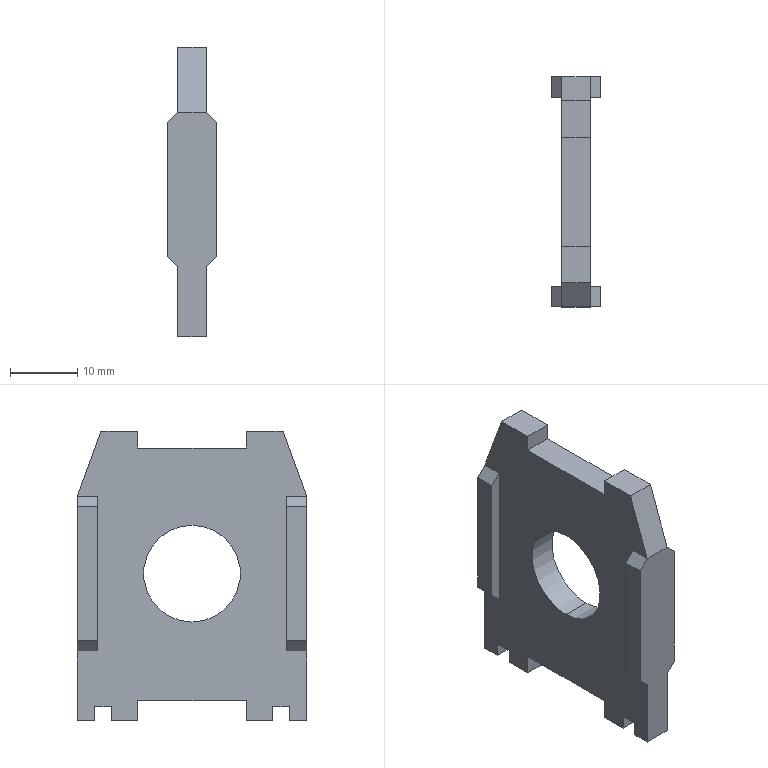Part | STEP file | 11-GY_Y300T-A_SCREW-30-V10-22111.11 | 1 solid | 42 faces | box 7.2 x 34.2 x 43.1 mm | volume 5332 mm3 | plane 40 | cylinder 2 | commonest cylinder face diameters 14.4 x2
STEP:
#1=CARTESIAN_POINT('',(-2.1,0.,7.2));
#2=VERTEX_POINT('',#1);
#3=CARTESIAN_POINT('',(-2.1,0.,-7.2));
#4=VERTEX_POINT('',#3);
#5=CARTESIAN_POINT('',(-2.1,0.,0.));
#6=DIRECTION('',(1.,0.,0.));
#7=DIRECTION('',(0.,0.,-1.));
#8=AXIS2_PLACEMENT_3D('',#5,#6,#7);
#9=CIRCLE('',#8,7.2);
#10=EDGE_CURVE('',#2,#4,#9,.T.);
#11=ORIENTED_EDGE('',*,*,#10,.F.);
#12=CARTESIAN_POINT('',(2.1,0.,7.2));
#13=VERTEX_POINT('',#12);
#14=CARTESIAN_POINT('',(2.1,0.,7.2));
#15=DIRECTION('',(1.,0.,0.));
#16=VECTOR('',#15,1000.);
#17=LINE('',#14,#16);
#18=EDGE_CURVE('',#2,#13,#17,.T.);
#19=ORIENTED_EDGE('',*,*,#18,.T.);
#20=CARTESIAN_POINT('',(2.1,0.,-7.2));
#21=VERTEX_POINT('',#20);
#22=CARTESIAN_POINT('',(2.1,0.,0.));
#23=DIRECTION('',(-1.,0.,0.));
#24=DIRECTION('',(0.,0.,-1.));
#25=AXIS2_PLACEMENT_3D('',#22,#23,#24);
#26=CIRCLE('',#25,7.2);
#27=EDGE_CURVE('',#21,#13,#26,.T.);
#28=ORIENTED_EDGE('',*,*,#27,.F.);
#29=CARTESIAN_POINT('',(2.1,0.,-7.2));
#30=DIRECTION('',(1.,0.,0.));
#31=VECTOR('',#30,1000.);
#32=LINE('',#29,#31);
#33=EDGE_CURVE('',#4,#21,#32,.T.);
#34=ORIENTED_EDGE('',*,*,#33,.F.);
#35=EDGE_LOOP('',(#11,#19,#28,#34));
#36=FACE_OUTER_BOUND('',#35,.T.);
#37=CARTESIAN_POINT('',(2.1,0.,0.));
#38=DIRECTION('',(1.,0.,0.));
#39=DIRECTION('',(0.,0.,-1.));
#40=AXIS2_PLACEMENT_3D('',#37,#38,#39);
#41=CYLINDRICAL_SURFACE('',#40,7.2);
#42=ADVANCED_FACE('',(#36),#41,.F.);
#43=CARTESIAN_POINT('',(2.1,-8.1,18.7));
#44=VERTEX_POINT('',#43);
#45=CARTESIAN_POINT('',(2.1,-8.1,21.2));
#46=VERTEX_POINT('',#45);
#47=CARTESIAN_POINT('',(2.1,-8.1,0.));
#48=DIRECTION('',(0.,0.,1.));
#49=VECTOR('',#48,1000.);
#50=LINE('',#47,#49);
#51=EDGE_CURVE('',#44,#46,#50,.T.);
#52=ORIENTED_EDGE('',*,*,#51,.T.);
#53=CARTESIAN_POINT('',(2.1,-13.569,21.2));
#54=VERTEX_POINT('',#53);
#55=CARTESIAN_POINT('',(2.1,0.,21.2));
#56=DIRECTION('',(0.,-1.,0.));
#57=VECTOR('',#56,1000.);
#58=LINE('',#55,#57);
#59=EDGE_CURVE('',#46,#54,#58,.T.);
#60=ORIENTED_EDGE('',*,*,#59,.T.);
#61=CARTESIAN_POINT('',(2.1,-17.1,11.5));
#62=VERTEX_POINT('',#61);
#63=CARTESIAN_POINT('',(2.1,-13.569,21.2));
#64=DIRECTION('',(0.,-0.342,-0.9397));
#65=VECTOR('',#64,1000.);
#66=LINE('',#63,#65);
#67=EDGE_CURVE('',#54,#62,#66,.T.);
#68=ORIENTED_EDGE('',*,*,#67,.T.);
#69=CARTESIAN_POINT('',(2.1,-14.1,11.5));
#70=VERTEX_POINT('',#69);
#71=CARTESIAN_POINT('',(2.1,0.,11.5));
#72=DIRECTION('',(0.,1.,0.));
#73=VECTOR('',#72,1000.);
#74=LINE('',#71,#73);
#75=EDGE_CURVE('',#62,#70,#74,.T.);
#76=ORIENTED_EDGE('',*,*,#75,.T.);
#77=CARTESIAN_POINT('',(2.1,-14.1,-11.5));
#78=VERTEX_POINT('',#77);
#79=CARTESIAN_POINT('',(2.1,-14.1,0.));
#80=DIRECTION('',(0.,0.,-1.));
#81=VECTOR('',#80,1000.);
#82=LINE('',#79,#81);
#83=EDGE_CURVE('',#70,#78,#82,.T.);
#84=ORIENTED_EDGE('',*,*,#83,.T.);
#85=CARTESIAN_POINT('',(2.1,-17.1,-11.5));
#86=VERTEX_POINT('',#85);
#87=CARTESIAN_POINT('',(2.1,0.,-11.5));
#88=DIRECTION('',(0.,-1.,0.));
#89=VECTOR('',#88,1000.);
#90=LINE('',#87,#89);
#91=EDGE_CURVE('',#78,#86,#90,.T.);
#92=ORIENTED_EDGE('',*,*,#91,.T.);
#93=CARTESIAN_POINT('',(2.1,-17.1,-21.9));
#94=VERTEX_POINT('',#93);
#95=CARTESIAN_POINT('',(2.1,-17.1,0.));
#96=DIRECTION('',(0.,0.,-1.));
#97=VECTOR('',#96,1000.);
#98=LINE('',#95,#97);
#99=EDGE_CURVE('',#86,#94,#98,.T.);
#100=ORIENTED_EDGE('',*,*,#99,.T.);
#101=CARTESIAN_POINT('',(2.1,-14.5,-21.9));
#102=VERTEX_POINT('',#101);
#103=CARTESIAN_POINT('',(2.1,0.,-21.9));
#104=DIRECTION('',(0.,1.,0.));
#105=VECTOR('',#104,1000.);
#106=LINE('',#103,#105);
#107=EDGE_CURVE('',#94,#102,#106,.T.);
#108=ORIENTED_EDGE('',*,*,#107,.T.);
#109=CARTESIAN_POINT('',(2.1,-14.5,-19.8));
#110=VERTEX_POINT('',#109);
#111=CARTESIAN_POINT('',(2.1,-14.5,0.));
#112=DIRECTION('',(0.,0.,1.));
#113=VECTOR('',#112,1000.);
#114=LINE('',#111,#113);
#115=EDGE_CURVE('',#102,#110,#114,.T.);
#116=ORIENTED_EDGE('',*,*,#115,.T.);
#117=CARTESIAN_POINT('',(2.1,-12.,-19.8));
#118=VERTEX_POINT('',#117);
#119=CARTESIAN_POINT('',(2.1,0.,-19.8));
#120=DIRECTION('',(0.,1.,0.));
#121=VECTOR('',#120,1000.);
#122=LINE('',#119,#121);
#123=EDGE_CURVE('',#110,#118,#122,.T.);
#124=ORIENTED_EDGE('',*,*,#123,.T.);
#125=CARTESIAN_POINT('',(2.1,-12.,-21.9));
#126=VERTEX_POINT('',#125);
#127=CARTESIAN_POINT('',(2.1,-12.,0.));
#128=DIRECTION('',(0.,0.,-1.));
#129=VECTOR('',#128,1000.);
#130=LINE('',#127,#129);
#131=EDGE_CURVE('',#118,#126,#130,.T.);
#132=ORIENTED_EDGE('',*,*,#131,.T.);
#133=CARTESIAN_POINT('',(2.1,-8.1,-21.9));
#134=VERTEX_POINT('',#133);
#135=CARTESIAN_POINT('',(2.1,0.,-21.9));
#136=DIRECTION('',(0.,1.,0.));
#137=VECTOR('',#136,1000.);
#138=LINE('',#135,#137);
#139=EDGE_CURVE('',#126,#134,#138,.T.);
#140=ORIENTED_EDGE('',*,*,#139,.T.);
#141=CARTESIAN_POINT('',(2.1,-8.1,-18.9));
#142=VERTEX_POINT('',#141);
#143=CARTESIAN_POINT('',(2.1,-8.1,0.));
#144=DIRECTION('',(0.,0.,1.));
#145=VECTOR('',#144,1000.);
#146=LINE('',#143,#145);
#147=EDGE_CURVE('',#134,#142,#146,.T.);
#148=ORIENTED_EDGE('',*,*,#147,.T.);
#149=CARTESIAN_POINT('',(2.1,8.1,-18.9));
#150=VERTEX_POINT('',#149);
#151=CARTESIAN_POINT('',(2.1,0.,-18.9));
#152=DIRECTION('',(0.,1.,0.));
#153=VECTOR('',#152,1000.);
#154=LINE('',#151,#153);
#155=EDGE_CURVE('',#142,#150,#154,.T.);
#156=ORIENTED_EDGE('',*,*,#155,.T.);
#157=CARTESIAN_POINT('',(2.1,8.1,-21.9));
#158=VERTEX_POINT('',#157);
#159=CARTESIAN_POINT('',(2.1,8.1,0.));
#160=DIRECTION('',(0.,0.,-1.));
#161=VECTOR('',#160,1000.);
#162=LINE('',#159,#161);
#163=EDGE_CURVE('',#150,#158,#162,.T.);
#164=ORIENTED_EDGE('',*,*,#163,.T.);
#165=CARTESIAN_POINT('',(2.1,12.,-21.9));
#166=VERTEX_POINT('',#165);
#167=CARTESIAN_POINT('',(2.1,0.,-21.9));
#168=DIRECTION('',(0.,1.,0.));
#169=VECTOR('',#168,1000.);
#170=LINE('',#167,#169);
#171=EDGE_CURVE('',#158,#166,#170,.T.);
#172=ORIENTED_EDGE('',*,*,#171,.T.);
#173=CARTESIAN_POINT('',(2.1,12.,-19.8));
#174=VERTEX_POINT('',#173);
#175=CARTESIAN_POINT('',(2.1,12.,0.));
#176=DIRECTION('',(0.,0.,1.));
#177=VECTOR('',#176,1000.);
#178=LINE('',#175,#177);
#179=EDGE_CURVE('',#166,#174,#178,.T.);
#180=ORIENTED_EDGE('',*,*,#179,.T.);
#181=CARTESIAN_POINT('',(2.1,14.5,-19.8));
#182=VERTEX_POINT('',#181);
#183=CARTESIAN_POINT('',(2.1,0.,-19.8));
#184=DIRECTION('',(0.,1.,0.));
#185=VECTOR('',#184,1000.);
#186=LINE('',#183,#185);
#187=EDGE_CURVE('',#174,#182,#186,.T.);
#188=ORIENTED_EDGE('',*,*,#187,.T.);
#189=CARTESIAN_POINT('',(2.1,14.5,-21.9));
#190=VERTEX_POINT('',#189);
#191=CARTESIAN_POINT('',(2.1,14.5,0.));
#192=DIRECTION('',(0.,0.,-1.));
#193=VECTOR('',#192,1000.);
#194=LINE('',#191,#193);
#195=EDGE_CURVE('',#182,#190,#194,.T.);
#196=ORIENTED_EDGE('',*,*,#195,.T.);
#197=CARTESIAN_POINT('',(2.1,17.1,-21.9));
#198=VERTEX_POINT('',#197);
#199=CARTESIAN_POINT('',(2.1,0.,-21.9));
#200=DIRECTION('',(0.,1.,0.));
#201=VECTOR('',#200,1000.);
#202=LINE('',#199,#201);
#203=EDGE_CURVE('',#190,#198,#202,.T.);
#204=ORIENTED_EDGE('',*,*,#203,.T.);
#205=CARTESIAN_POINT('',(2.1,17.1,-11.5));
#206=VERTEX_POINT('',#205);
#207=CARTESIAN_POINT('',(2.1,17.1,0.));
#208=DIRECTION('',(0.,0.,1.));
#209=VECTOR('',#208,1000.);
#210=LINE('',#207,#209);
#211=EDGE_CURVE('',#198,#206,#210,.T.);
#212=ORIENTED_EDGE('',*,*,#211,.T.);
#213=CARTESIAN_POINT('',(2.1,14.1,-11.5));
#214=VERTEX_POINT('',#213);
#215=CARTESIAN_POINT('',(2.1,0.,-11.5));
#216=DIRECTION('',(0.,-1.,0.));
#217=VECTOR('',#216,1000.);
#218=LINE('',#215,#217);
#219=EDGE_CURVE('',#206,#214,#218,.T.);
#220=ORIENTED_EDGE('',*,*,#219,.T.);
#221=CARTESIAN_POINT('',(2.1,14.1,11.5));
#222=VERTEX_POINT('',#221);
#223=CARTESIAN_POINT('',(2.1,14.1,0.));
#224=DIRECTION('',(0.,0.,1.));
#225=VECTOR('',#224,1000.);
#226=LINE('',#223,#225);
#227=EDGE_CURVE('',#214,#222,#226,.T.);
#228=ORIENTED_EDGE('',*,*,#227,.T.);
#229=CARTESIAN_POINT('',(2.1,17.1,11.5));
#230=VERTEX_POINT('',#229);
#231=CARTESIAN_POINT('',(2.1,0.,11.5));
#232=DIRECTION('',(0.,1.,0.));
#233=VECTOR('',#232,1000.);
#234=LINE('',#231,#233);
#235=EDGE_CURVE('',#222,#230,#234,.T.);
#236=ORIENTED_EDGE('',*,*,#235,.T.);
#237=CARTESIAN_POINT('',(2.1,13.569,21.2));
#238=VERTEX_POINT('',#237);
#239=CARTESIAN_POINT('',(2.1,17.1,11.5));
#240=DIRECTION('',(0.,-0.342,0.9397));
#241=VECTOR('',#240,1000.);
#242=LINE('',#239,#241);
#243=EDGE_CURVE('',#230,#238,#242,.T.);
#244=ORIENTED_EDGE('',*,*,#243,.T.);
#245=CARTESIAN_POINT('',(2.1,8.1,21.2));
#246=VERTEX_POINT('',#245);
#247=CARTESIAN_POINT('',(2.1,0.,21.2));
#248=DIRECTION('',(0.,-1.,0.));
#249=VECTOR('',#248,1000.);
#250=LINE('',#247,#249);
#251=EDGE_CURVE('',#238,#246,#250,.T.);
#252=ORIENTED_EDGE('',*,*,#251,.T.);
#253=CARTESIAN_POINT('',(2.1,8.1,18.7));
#254=VERTEX_POINT('',#253);
#255=CARTESIAN_POINT('',(2.1,8.1,0.));
#256=DIRECTION('',(0.,0.,-1.));
#257=VECTOR('',#256,1000.);
#258=LINE('',#255,#257);
#259=EDGE_CURVE('',#246,#254,#258,.T.);
#260=ORIENTED_EDGE('',*,*,#259,.T.);
#261=CARTESIAN_POINT('',(2.1,0.,18.7));
#262=DIRECTION('',(0.,-1.,0.));
#263=VECTOR('',#262,1000.);
#264=LINE('',#261,#263);
#265=EDGE_CURVE('',#254,#44,#264,.T.);
#266=ORIENTED_EDGE('',*,*,#265,.T.);
#267=EDGE_LOOP('',(#52,#60,#68,#76,#84,#92,#100,#108,#116,#124,#132,#140,#148,#156,#164,#172,#180,#188,#196,#204,#212,#220,#228,#236,#244,#252,#260,#266));
#268=FACE_OUTER_BOUND('',#267,.T.);
#269=ORIENTED_EDGE('',*,*,#27,.T.);
#270=CARTESIAN_POINT('',(2.1,0.,0.));
#271=DIRECTION('',(-1.,0.,0.));
#272=DIRECTION('',(0.,0.,-1.));
#273=AXIS2_PLACEMENT_3D('',#270,#271,#272);
#274=CIRCLE('',#273,7.2);
#275=EDGE_CURVE('',#13,#21,#274,.T.);
#276=ORIENTED_EDGE('',*,*,#275,.T.);
#277=EDGE_LOOP('',(#269,#276));
#278=FACE_BOUND('',#277,.T.);
#279=CARTESIAN_POINT('',(2.1,0.,0.));
#280=DIRECTION('',(1.,0.,0.));
#281=DIRECTION('',(0.,0.,-1.));
#282=AXIS2_PLACEMENT_3D('',#279,#280,#281);
#283=PLANE('',#282);
#284=ADVANCED_FACE('',(#268,#278),#283,.T.);
#285=CARTESIAN_POINT('',(-2.1,-13.569,21.2));
#286=VERTEX_POINT('',#285);
#287=CARTESIAN_POINT('',(2.1,-13.569,21.2));
#288=DIRECTION('',(-1.,0.,0.));
#289=VECTOR('',#288,1000.);
#290=LINE('',#287,#289);
#291=EDGE_CURVE('',#54,#286,#290,.T.);
#292=ORIENTED_EDGE('',*,*,#291,.F.);
#293=ORIENTED_EDGE('',*,*,#59,.F.);
#294=CARTESIAN_POINT('',(-2.1,-8.1,21.2));
#295=VERTEX_POINT('',#294);
#296=CARTESIAN_POINT('',(2.1,-8.1,21.2));
#297=DIRECTION('',(1.,0.,0.));
#298=VECTOR('',#297,1000.);
#299=LINE('',#296,#298);
#300=EDGE_CURVE('',#295,#46,#299,.T.);
#301=ORIENTED_EDGE('',*,*,#300,.F.);
#302=CARTESIAN_POINT('',(-2.1,-8.1,21.2));
#303=DIRECTION('',(0.,1.,0.));
#304=VECTOR('',#303,1000.);
#305=LINE('',#302,#304);
#306=EDGE_CURVE('',#286,#295,#305,.T.);
#307=ORIENTED_EDGE('',*,*,#306,.F.);
#308=EDGE_LOOP('',(#292,#293,#301,#307));
#309=FACE_OUTER_BOUND('',#308,.T.);
#310=CARTESIAN_POINT('',(2.1,-8.1,21.2));
#311=DIRECTION('',(0.,0.,-1.));
#312=DIRECTION('',(-1.,0.,0.));
#313=AXIS2_PLACEMENT_3D('',#310,#311,#312);
#314=PLANE('',#313);
#315=ADVANCED_FACE('',(#309),#314,.F.);
#316=ORIENTED_EDGE('',*,*,#300,.T.);
#317=ORIENTED_EDGE('',*,*,#51,.F.);
#318=CARTESIAN_POINT('',(-2.1,-8.1,18.7));
#319=VERTEX_POINT('',#318);
#320=CARTESIAN_POINT('',(2.1,-8.1,18.7));
#321=DIRECTION('',(1.,0.,0.));
#322=VECTOR('',#321,1000.);
#323=LINE('',#320,#322);
#324=EDGE_CURVE('',#319,#44,#323,.T.);
#325=ORIENTED_EDGE('',*,*,#324,.F.);
#326=CARTESIAN_POINT('',(-2.1,-8.1,18.7));
#327=DIRECTION('',(0.,0.,-1.));
#328=VECTOR('',#327,1000.);
#329=LINE('',#326,#328);
#330=EDGE_CURVE('',#295,#319,#329,.T.);
#331=ORIENTED_EDGE('',*,*,#330,.F.);
#332=EDGE_LOOP('',(#316,#317,#325,#331));
#333=FACE_OUTER_BOUND('',#332,.T.);
#334=CARTESIAN_POINT('',(2.1,-8.1,18.7));
#335=DIRECTION('',(0.,-1.,0.));
#336=DIRECTION('',(0.,0.,-1.));
#337=AXIS2_PLACEMENT_3D('',#334,#335,#336);
#338=PLANE('',#337);
#339=ADVANCED_FACE('',(#333),#338,.F.);
#340=ORIENTED_EDGE('',*,*,#324,.T.);
#341=ORIENTED_EDGE('',*,*,#265,.F.);
#342=CARTESIAN_POINT('',(-2.1,8.1,18.7));
#343=VERTEX_POINT('',#342);
#344=CARTESIAN_POINT('',(2.1,8.1,18.7));
#345=DIRECTION('',(1.,0.,0.));
#346=VECTOR('',#345,1000.);
#347=LINE('',#344,#346);
#348=EDGE_CURVE('',#343,#254,#347,.T.);
#349=ORIENTED_EDGE('',*,*,#348,.F.);
#350=CARTESIAN_POINT('',(-2.1,8.1,18.7));
#351=DIRECTION('',(0.,1.,0.));
#352=VECTOR('',#351,1000.);
#353=LINE('',#350,#352);
#354=EDGE_CURVE('',#319,#343,#353,.T.);
#355=ORIENTED_EDGE('',*,*,#354,.F.);
#356=EDGE_LOOP('',(#340,#341,#349,#355));
#357=FACE_OUTER_BOUND('',#356,.T.);
#358=CARTESIAN_POINT('',(2.1,8.1,18.7));
#359=DIRECTION('',(0.,0.,-1.));
#360=DIRECTION('',(-1.,0.,0.));
#361=AXIS2_PLACEMENT_3D('',#358,#359,#360);
#362=PLANE('',#361);
#363=ADVANCED_FACE('',(#357),#362,.F.);
#364=ORIENTED_EDGE('',*,*,#348,.T.);
#365=ORIENTED_EDGE('',*,*,#259,.F.);
#366=CARTESIAN_POINT('',(-2.1,8.1,21.2));
#367=VERTEX_POINT('',#366);
#368=CARTESIAN_POINT('',(2.1,8.1,21.2));
#369=DIRECTION('',(1.,0.,0.));
#370=VECTOR('',#369,1000.);
#371=LINE('',#368,#370);
#372=EDGE_CURVE('',#367,#246,#371,.T.);
#373=ORIENTED_EDGE('',*,*,#372,.F.);
#374=CARTESIAN_POINT('',(-2.1,8.1,21.2));
#375=DIRECTION('',(0.,0.,1.));
#376=VECTOR('',#375,1000.);
#377=LINE('',#374,#376);
#378=EDGE_CURVE('',#343,#367,#377,.T.);
#379=ORIENTED_EDGE('',*,*,#378,.F.);
#380=EDGE_LOOP('',(#364,#365,#373,#379));
#381=FACE_OUTER_BOUND('',#380,.T.);
#382=CARTESIAN_POINT('',(2.1,8.1,21.2));
#383=DIRECTION('',(0.,1.,0.));
#384=DIRECTION('',(0.,0.,1.));
#385=AXIS2_PLACEMENT_3D('',#382,#383,#384);
#386=PLANE('',#385);
#387=ADVANCED_FACE('',(#381),#386,.F.);
#388=ORIENTED_EDGE('',*,*,#372,.T.);
#389=ORIENTED_EDGE('',*,*,#251,.F.);
#390=CARTESIAN_POINT('',(-2.1,13.569,21.2));
#391=VERTEX_POINT('',#390);
#392=CARTESIAN_POINT('',(2.1,13.569,21.2));
#393=DIRECTION('',(1.,0.,0.));
#394=VECTOR('',#393,1000.);
#395=LINE('',#392,#394);
#396=EDGE_CURVE('',#391,#238,#395,.T.);
#397=ORIENTED_EDGE('',*,*,#396,.F.);
#398=CARTESIAN_POINT('',(-2.1,13.569,21.2));
#399=DIRECTION('',(0.,1.,0.));
#400=VECTOR('',#399,1000.);
#401=LINE('',#398,#400);
#402=EDGE_CURVE('',#367,#391,#401,.T.);
#403=ORIENTED_EDGE('',*,*,#402,.F.);
#404=EDGE_LOOP('',(#388,#389,#397,#403));
#405=FACE_OUTER_BOUND('',#404,.T.);
#406=CARTESIAN_POINT('',(2.1,13.569,21.2));
#407=DIRECTION('',(0.,0.,-1.));
#408=DIRECTION('',(-1.,0.,0.));
#409=AXIS2_PLACEMENT_3D('',#406,#407,#408);
#410=PLANE('',#409);
#411=ADVANCED_FACE('',(#405),#410,.F.);
#412=ORIENTED_EDGE('',*,*,#396,.T.);
#413=ORIENTED_EDGE('',*,*,#243,.F.);
#414=CARTESIAN_POINT('',(-2.1,17.1,11.5));
#415=VERTEX_POINT('',#414);
#416=CARTESIAN_POINT('',(2.1,17.1,11.5));
#417=DIRECTION('',(1.,0.,0.));
#418=VECTOR('',#417,1000.);
#419=LINE('',#416,#418);
#420=EDGE_CURVE('',#415,#230,#419,.T.);
#421=ORIENTED_EDGE('',*,*,#420,.F.);
#422=CARTESIAN_POINT('',(-2.1,17.1,11.5));
#423=DIRECTION('',(0.,0.342,-0.9397));
#424=VECTOR('',#423,1000.);
#425=LINE('',#422,#424);
#426=EDGE_CURVE('',#391,#415,#425,.T.);
#427=ORIENTED_EDGE('',*,*,#426,.F.);
#428=EDGE_LOOP('',(#412,#413,#421,#427));
#429=FACE_OUTER_BOUND('',#428,.T.);
#430=CARTESIAN_POINT('',(2.1,17.1,11.5));
#431=DIRECTION('',(0.,-0.9397,-0.342));
#432=DIRECTION('',(0.,0.342,-0.9397));
#433=AXIS2_PLACEMENT_3D('',#430,#431,#432);
#434=PLANE('',#433);
#435=ADVANCED_FACE('',(#429),#434,.F.);
#436=CARTESIAN_POINT('',(3.6,14.1,10.));
#437=VERTEX_POINT('',#436);
#438=CARTESIAN_POINT('',(2.1,14.1,11.5));
#439=DIRECTION('',(0.7071,0.,-0.7071));
#440=VECTOR('',#439,1000.);
#441=LINE('',#438,#440);
#442=EDGE_CURVE('',#222,#437,#441,.T.);
#443=ORIENTED_EDGE('',*,*,#442,.T.);
#444=CARTESIAN_POINT('',(3.6,17.1,10.));
#445=VERTEX_POINT('',#444);
#446=CARTESIAN_POINT('',(3.6,14.1,10.));
#447=DIRECTION('',(0.,1.,0.));
#448=VECTOR('',#447,1000.);
#449=LINE('',#446,#448);
#450=EDGE_CURVE('',#437,#445,#449,.T.);
#451=ORIENTED_EDGE('',*,*,#450,.T.);
#452=CARTESIAN_POINT('',(2.1,17.1,11.5));
#453=DIRECTION('',(-0.7071,0.,0.7071));
#454=VECTOR('',#453,1000.);
#455=LINE('',#452,#454);
#456=EDGE_CURVE('',#445,#230,#455,.T.);
#457=ORIENTED_EDGE('',*,*,#456,.T.);
#458=ORIENTED_EDGE('',*,*,#235,.F.);
#459=EDGE_LOOP('',(#443,#451,#457,#458));
#460=FACE_OUTER_BOUND('',#459,.T.);
#461=CARTESIAN_POINT('',(2.1,14.1,11.5));
#462=DIRECTION('',(0.7071,0.,0.7071));
#463=DIRECTION('',(0.7071,0.,-0.7071));
#464=AXIS2_PLACEMENT_3D('',#461,#462,#463);
#465=PLANE('',#464);
#466=ADVANCED_FACE('',(#460),#465,.T.);
#467=CARTESIAN_POINT('',(3.6,14.1,-10.));
#468=VERTEX_POINT('',#467);
#469=CARTESIAN_POINT('',(3.6,14.1,-10.));
#470=DIRECTION('',(-0.7071,0.,-0.7071));
#471=VECTOR('',#470,1000.);
#472=LINE('',#469,#471);
#473=EDGE_CURVE('',#468,#214,#472,.T.);
#474=ORIENTED_EDGE('',*,*,#473,.F.);
#475=CARTESIAN_POINT('',(3.6,14.1,0.));
#476=DIRECTION('',(0.,0.,-1.));
#477=VECTOR('',#476,1000.);
#478=LINE('',#475,#477);
#479=EDGE_CURVE('',#437,#468,#478,.T.);
#480=ORIENTED_EDGE('',*,*,#479,.F.);
#481=ORIENTED_EDGE('',*,*,#442,.F.);
#482=ORIENTED_EDGE('',*,*,#227,.F.);
#483=EDGE_LOOP('',(#474,#480,#481,#482));
#484=FACE_OUTER_BOUND('',#483,.T.);
#485=CARTESIAN_POINT('',(0.,14.1,0.));
#486=DIRECTION('',(0.,1.,0.));
#487=DIRECTION('',(0.,0.,1.));
#488=AXIS2_PLACEMENT_3D('',#485,#486,#487);
#489=PLANE('',#488);
#490=ADVANCED_FACE('',(#484),#489,.F.);
#491=ORIENTED_EDGE('',*,*,#473,.T.);
#492=ORIENTED_EDGE('',*,*,#219,.F.);
#493=CARTESIAN_POINT('',(3.6,17.1,-10.));
#494=VERTEX_POINT('',#493);
#495=CARTESIAN_POINT('',(3.6,17.1,-10.));
#496=DIRECTION('',(0.7071,0.,0.7071));
#497=VECTOR('',#496,1000.);
#498=LINE('',#495,#497);
#499=EDGE_CURVE('',#206,#494,#498,.T.);
#500=ORIENTED_EDGE('',*,*,#499,.T.);
#501=CARTESIAN_POINT('',(3.6,14.1,-10.));
#502=DIRECTION('',(0.,-1.,0.));
#503=VECTOR('',#502,1000.);
#504=LINE('',#501,#503);
#505=EDGE_CURVE('',#494,#468,#504,.T.);
#506=ORIENTED_EDGE('',*,*,#505,.T.);
#507=EDGE_LOOP('',(#491,#492,#500,#506));
#508=FACE_OUTER_BOUND('',#507,.T.);
#509=CARTESIAN_POINT('',(3.6,14.1,-10.));
#510=DIRECTION('',(0.7071,0.,-0.7071));
#511=DIRECTION('',(-0.7071,0.,-0.7071));
#512=AXIS2_PLACEMENT_3D('',#509,#510,#511);
#513=PLANE('',#512);
#514=ADVANCED_FACE('',(#508),#513,.T.);
#515=CARTESIAN_POINT('',(-3.6,17.1,-10.));
#516=VERTEX_POINT('',#515);
#517=CARTESIAN_POINT('',(-2.1,17.1,-11.5));
#518=VERTEX_POINT('',#517);
#519=CARTESIAN_POINT('',(-3.6,17.1,-10.));
#520=DIRECTION('',(0.7071,0.,-0.7071));
#521=VECTOR('',#520,1000.);
#522=LINE('',#519,#521);
#523=EDGE_CURVE('',#516,#518,#522,.T.);
#524=ORIENTED_EDGE('',*,*,#523,.F.);
#525=CARTESIAN_POINT('',(-3.6,17.1,10.));
#526=VERTEX_POINT('',#525);
#527=CARTESIAN_POINT('',(-3.6,17.1,-21.9));
#528=DIRECTION('',(0.,0.,-1.));
#529=VECTOR('',#528,1000.);
#530=LINE('',#527,#529);
#531=EDGE_CURVE('',#526,#516,#530,.T.);
#532=ORIENTED_EDGE('',*,*,#531,.F.);
#533=CARTESIAN_POINT('',(-2.1,17.1,11.5));
#534=DIRECTION('',(-0.7071,0.,-0.7071));
#535=VECTOR('',#534,1000.);
#536=LINE('',#533,#535);
#537=EDGE_CURVE('',#415,#526,#536,.T.);
#538=ORIENTED_EDGE('',*,*,#537,.F.);
#539=ORIENTED_EDGE('',*,*,#420,.T.);
#540=ORIENTED_EDGE('',*,*,#456,.F.);
#541=CARTESIAN_POINT('',(3.6,17.1,-21.9));
#542=DIRECTION('',(0.,0.,1.));
#543=VECTOR('',#542,1000.);
#544=LINE('',#541,#543);
#545=EDGE_CURVE('',#494,#445,#544,.T.);
#546=ORIENTED_EDGE('',*,*,#545,.F.);
#547=ORIENTED_EDGE('',*,*,#499,.F.);
#548=ORIENTED_EDGE('',*,*,#211,.F.);
#549=CARTESIAN_POINT('',(-2.1,17.1,-21.9));
#550=VERTEX_POINT('',#549);
#551=CARTESIAN_POINT('',(2.1,17.1,-21.9));
#552=DIRECTION('',(1.,0.,0.));
#553=VECTOR('',#552,1000.);
#554=LINE('',#551,#553);
#555=EDGE_CURVE('',#550,#198,#554,.T.);
#556=ORIENTED_EDGE('',*,*,#555,.F.);
#557=CARTESIAN_POINT('',(-2.1,17.1,-21.9));
#558=DIRECTION('',(0.,0.,-1.));
#559=VECTOR('',#558,1000.);
#560=LINE('',#557,#559);
#561=EDGE_CURVE('',#518,#550,#560,.T.);
#562=ORIENTED_EDGE('',*,*,#561,.F.);
#563=EDGE_LOOP('',(#524,#532,#538,#539,#540,#546,#547,#548,#556,#562));
#564=FACE_OUTER_BOUND('',#563,.T.);
#565=CARTESIAN_POINT('',(2.1,17.1,-21.9));
#566=DIRECTION('',(0.,-1.,0.));
#567=DIRECTION('',(0.,0.,-1.));
#568=AXIS2_PLACEMENT_3D('',#565,#566,#567);
#569=PLANE('',#568);
#570=ADVANCED_FACE('',(#564),#569,.F.);
#571=ORIENTED_EDGE('',*,*,#555,.T.);
#572=ORIENTED_EDGE('',*,*,#203,.F.);
#573=CARTESIAN_POINT('',(-2.1,14.5,-21.9));
#574=VERTEX_POINT('',#573);
#575=CARTESIAN_POINT('',(2.1,14.5,-21.9));
#576=DIRECTION('',(1.,0.,0.));
#577=VECTOR('',#576,1000.);
#578=LINE('',#575,#577);
#579=EDGE_CURVE('',#574,#190,#578,.T.);
#580=ORIENTED_EDGE('',*,*,#579,.F.);
#581=CARTESIAN_POINT('',(-2.1,14.5,-21.9));
#582=DIRECTION('',(0.,-1.,0.));
#583=VECTOR('',#582,1000.);
#584=LINE('',#581,#583);
#585=EDGE_CURVE('',#550,#574,#584,.T.);
#586=ORIENTED_EDGE('',*,*,#585,.F.);
#587=EDGE_LOOP('',(#571,#572,#580,#586));
#588=FACE_OUTER_BOUND('',#587,.T.);
#589=CARTESIAN_POINT('',(2.1,14.5,-21.9));
#590=DIRECTION('',(0.,0.,1.));
#591=DIRECTION('',(1.,0.,0.));
#592=AXIS2_PLACEMENT_3D('',#589,#590,#591);
#593=PLANE('',#592);
#594=ADVANCED_FACE('',(#588),#593,.F.);
#595=ORIENTED_EDGE('',*,*,#579,.T.);
#596=ORIENTED_EDGE('',*,*,#195,.F.);
#597=CARTESIAN_POINT('',(-2.1,14.5,-19.8));
#598=VERTEX_POINT('',#597);
#599=CARTESIAN_POINT('',(2.1,14.5,-19.8));
#600=DIRECTION('',(1.,0.,0.));
#601=VECTOR('',#600,1000.);
#602=LINE('',#599,#601);
#603=EDGE_CURVE('',#598,#182,#602,.T.);
#604=ORIENTED_EDGE('',*,*,#603,.F.);
#605=CARTESIAN_POINT('',(-2.1,14.5,-19.8));
#606=DIRECTION('',(0.,0.,1.));
#607=VECTOR('',#606,1000.);
#608=LINE('',#605,#607);
#609=EDGE_CURVE('',#574,#598,#608,.T.);
#610=ORIENTED_EDGE('',*,*,#609,.F.);
#611=EDGE_LOOP('',(#595,#596,#604,#610));
#612=FACE_OUTER_BOUND('',#611,.T.);
#613=CARTESIAN_POINT('',(2.1,14.5,-19.8));
#614=DIRECTION('',(0.,1.,0.));
#615=DIRECTION('',(0.,0.,1.));
#616=AXIS2_PLACEMENT_3D('',#613,#614,#615);
#617=PLANE('',#616);
#618=ADVANCED_FACE('',(#612),#617,.F.);
#619=ORIENTED_EDGE('',*,*,#603,.T.);
#620=ORIENTED_EDGE('',*,*,#187,.F.);
#621=CARTESIAN_POINT('',(-2.1,12.,-19.8));
#622=VERTEX_POINT('',#621);
#623=CARTESIAN_POINT('',(2.1,12.,-19.8));
#624=DIRECTION('',(1.,0.,0.));
#625=VECTOR('',#624,1000.);
#626=LINE('',#623,#625);
#627=EDGE_CURVE('',#622,#174,#626,.T.);
#628=ORIENTED_EDGE('',*,*,#627,.F.);
#629=CARTESIAN_POINT('',(-2.1,12.,-19.8));
#630=DIRECTION('',(0.,-1.,0.));
#631=VECTOR('',#630,1000.);
#632=LINE('',#629,#631);
#633=EDGE_CURVE('',#598,#622,#632,.T.);
#634=ORIENTED_EDGE('',*,*,#633,.F.);
#635=EDGE_LOOP('',(#619,#620,#628,#634));
#636=FACE_OUTER_BOUND('',#635,.T.);
#637=CARTESIAN_POINT('',(2.1,12.,-19.8));
#638=DIRECTION('',(0.,0.,1.));
#639=DIRECTION('',(1.,0.,0.));
#640=AXIS2_PLACEMENT_3D('',#637,#638,#639);
#641=PLANE('',#640);
#642=ADVANCED_FACE('',(#636),#641,.F.);
#643=ORIENTED_EDGE('',*,*,#627,.T.);
#644=ORIENTED_EDGE('',*,*,#179,.F.);
#645=CARTESIAN_POINT('',(-2.1,12.,-21.9));
#646=VERTEX_POINT('',#645);
#647=CARTESIAN_POINT('',(2.1,12.,-21.9));
#648=DIRECTION('',(1.,0.,0.));
#649=VECTOR('',#648,1000.);
#650=LINE('',#647,#649);
#651=EDGE_CURVE('',#646,#166,#650,.T.);
#652=ORIENTED_EDGE('',*,*,#651,.F.);
#653=CARTESIAN_POINT('',(-2.1,12.,-21.9));
#654=DIRECTION('',(0.,0.,-1.));
#655=VECTOR('',#654,1000.);
#656=LINE('',#653,#655);
#657=EDGE_CURVE('',#622,#646,#656,.T.);
#658=ORIENTED_EDGE('',*,*,#657,.F.);
#659=EDGE_LOOP('',(#643,#644,#652,#658));
#660=FACE_OUTER_BOUND('',#659,.T.);
#661=CARTESIAN_POINT('',(2.1,12.,-21.9));
#662=DIRECTION('',(0.,-1.,0.));
#663=DIRECTION('',(0.,0.,-1.));
#664=AXIS2_PLACEMENT_3D('',#661,#662,#663);
#665=PLANE('',#664);
#666=ADVANCED_FACE('',(#660),#665,.F.);
#667=ORIENTED_EDGE('',*,*,#651,.T.);
#668=ORIENTED_EDGE('',*,*,#171,.F.);
#669=CARTESIAN_POINT('',(-2.1,8.1,-21.9));
#670=VERTEX_POINT('',#669);
#671=CARTESIAN_POINT('',(2.1,8.1,-21.9));
#672=DIRECTION('',(1.,0.,0.));
#673=VECTOR('',#672,1000.);
#674=LINE('',#671,#673);
#675=EDGE_CURVE('',#670,#158,#674,.T.);
#676=ORIENTED_EDGE('',*,*,#675,.F.);
#677=CARTESIAN_POINT('',(-2.1,8.1,-21.9));
#678=DIRECTION('',(0.,-1.,0.));
#679=VECTOR('',#678,1000.);
#680=LINE('',#677,#679);
#681=EDGE_CURVE('',#646,#670,#680,.T.);
#682=ORIENTED_EDGE('',*,*,#681,.F.);
#683=EDGE_LOOP('',(#667,#668,#676,#682));
#684=FACE_OUTER_BOUND('',#683,.T.);
#685=CARTESIAN_POINT('',(2.1,8.1,-21.9));
#686=DIRECTION('',(0.,0.,1.));
#687=DIRECTION('',(1.,0.,0.));
#688=AXIS2_PLACEMENT_3D('',#685,#686,#687);
#689=PLANE('',#688);
#690=ADVANCED_FACE('',(#684),#689,.F.);
#691=ORIENTED_EDGE('',*,*,#675,.T.);
#692=ORIENTED_EDGE('',*,*,#163,.F.);
#693=CARTESIAN_POINT('',(-2.1,8.1,-18.9));
#694=VERTEX_POINT('',#693);
#695=CARTESIAN_POINT('',(2.1,8.1,-18.9));
#696=DIRECTION('',(1.,0.,0.));
#697=VECTOR('',#696,1000.);
#698=LINE('',#695,#697);
#699=EDGE_CURVE('',#694,#150,#698,.T.);
#700=ORIENTED_EDGE('',*,*,#699,.F.);
#701=CARTESIAN_POINT('',(-2.1,8.1,-18.9));
#702=DIRECTION('',(0.,0.,1.));
#703=VECTOR('',#702,1000.);
#704=LINE('',#701,#703);
#705=EDGE_CURVE('',#670,#694,#704,.T.);
#706=ORIENTED_EDGE('',*,*,#705,.F.);
#707=EDGE_LOOP('',(#691,#692,#700,#706));
#708=FACE_OUTER_BOUND('',#707,.T.);
#709=CARTESIAN_POINT('',(2.1,8.1,-18.9));
#710=DIRECTION('',(0.,1.,0.));
#711=DIRECTION('',(0.,0.,1.));
#712=AXIS2_PLACEMENT_3D('',#709,#710,#711);
#713=PLANE('',#712);
#714=ADVANCED_FACE('',(#708),#713,.F.);
#715=ORIENTED_EDGE('',*,*,#699,.T.);
#716=ORIENTED_EDGE('',*,*,#155,.F.);
#717=CARTESIAN_POINT('',(-2.1,-8.1,-18.9));
#718=VERTEX_POINT('',#717);
#719=CARTESIAN_POINT('',(2.1,-8.1,-18.9));
#720=DIRECTION('',(1.,0.,0.));
#721=VECTOR('',#720,1000.);
#722=LINE('',#719,#721);
#723=EDGE_CURVE('',#718,#142,#722,.T.);
#724=ORIENTED_EDGE('',*,*,#723,.F.);
#725=CARTESIAN_POINT('',(-2.1,-8.1,-18.9));
#726=DIRECTION('',(0.,-1.,0.));
#727=VECTOR('',#726,1000.);
#728=LINE('',#725,#727);
#729=EDGE_CURVE('',#694,#718,#728,.T.);
#730=ORIENTED_EDGE('',*,*,#729,.F.);
#731=EDGE_LOOP('',(#715,#716,#724,#730));
#732=FACE_OUTER_BOUND('',#731,.T.);
#733=CARTESIAN_POINT('',(2.1,-8.1,-18.9));
#734=DIRECTION('',(0.,0.,1.));
#735=DIRECTION('',(1.,0.,0.));
#736=AXIS2_PLACEMENT_3D('',#733,#734,#735);
#737=PLANE('',#736);
#738=ADVANCED_FACE('',(#732),#737,.F.);
#739=ORIENTED_EDGE('',*,*,#723,.T.);
#740=ORIENTED_EDGE('',*,*,#147,.F.);
#741=CARTESIAN_POINT('',(-2.1,-8.1,-21.9));
#742=VERTEX_POINT('',#741);
#743=CARTESIAN_POINT('',(2.1,-8.1,-21.9));
#744=DIRECTION('',(1.,0.,0.));
#745=VECTOR('',#744,1000.);
#746=LINE('',#743,#745);
#747=EDGE_CURVE('',#742,#134,#746,.T.);
#748=ORIENTED_EDGE('',*,*,#747,.F.);
#749=CARTESIAN_POINT('',(-2.1,-8.1,-21.9));
#750=DIRECTION('',(0.,0.,-1.));
#751=VECTOR('',#750,1000.);
#752=LINE('',#749,#751);
#753=EDGE_CURVE('',#718,#742,#752,.T.);
#754=ORIENTED_EDGE('',*,*,#753,.F.);
#755=EDGE_LOOP('',(#739,#740,#748,#754));
#756=FACE_OUTER_BOUND('',#755,.T.);
#757=CARTESIAN_POINT('',(2.1,-8.1,-21.9));
#758=DIRECTION('',(0.,-1.,0.));
#759=DIRECTION('',(0.,0.,-1.));
#760=AXIS2_PLACEMENT_3D('',#757,#758,#759);
#761=PLANE('',#760);
#762=ADVANCED_FACE('',(#756),#761,.F.);
#763=ORIENTED_EDGE('',*,*,#747,.T.);
#764=ORIENTED_EDGE('',*,*,#139,.F.);
#765=CARTESIAN_POINT('',(-2.1,-12.,-21.9));
#766=VERTEX_POINT('',#765);
#767=CARTESIAN_POINT('',(2.1,-12.,-21.9));
#768=DIRECTION('',(1.,0.,0.));
#769=VECTOR('',#768,1000.);
#770=LINE('',#767,#769);
#771=EDGE_CURVE('',#766,#126,#770,.T.);
#772=ORIENTED_EDGE('',*,*,#771,.F.);
#773=CARTESIAN_POINT('',(-2.1,-12.,-21.9));
#774=DIRECTION('',(0.,-1.,0.));
#775=VECTOR('',#774,1000.);
#776=LINE('',#773,#775);
#777=EDGE_CURVE('',#742,#766,#776,.T.);
#778=ORIENTED_EDGE('',*,*,#777,.F.);
#779=EDGE_LOOP('',(#763,#764,#772,#778));
#780=FACE_OUTER_BOUND('',#779,.T.);
#781=CARTESIAN_POINT('',(2.1,-12.,-21.9));
#782=DIRECTION('',(0.,0.,1.));
#783=DIRECTION('',(1.,0.,0.));
#784=AXIS2_PLACEMENT_3D('',#781,#782,#783);
#785=PLANE('',#784);
#786=ADVANCED_FACE('',(#780),#785,.F.);
#787=ORIENTED_EDGE('',*,*,#771,.T.);
#788=ORIENTED_EDGE('',*,*,#131,.F.);
#789=CARTESIAN_POINT('',(-2.1,-12.,-19.8));
#790=VERTEX_POINT('',#789);
#791=CARTESIAN_POINT('',(2.1,-12.,-19.8));
#792=DIRECTION('',(1.,0.,0.));
#793=VECTOR('',#792,1000.);
#794=LINE('',#791,#793);
#795=EDGE_CURVE('',#790,#118,#794,.T.);
#796=ORIENTED_EDGE('',*,*,#795,.F.);
#797=CARTESIAN_POINT('',(-2.1,-12.,-19.8));
#798=DIRECTION('',(0.,0.,1.));
#799=VECTOR('',#798,1000.);
#800=LINE('',#797,#799);
#801=EDGE_CURVE('',#766,#790,#800,.T.);
#802=ORIENTED_EDGE('',*,*,#801,.F.);
#803=EDGE_LOOP('',(#787,#788,#796,#802));
#804=FACE_OUTER_BOUND('',#803,.T.);
#805=CARTESIAN_POINT('',(2.1,-12.,-19.8));
#806=DIRECTION('',(0.,1.,0.));
#807=DIRECTION('',(0.,0.,1.));
#808=AXIS2_PLACEMENT_3D('',#805,#806,#807);
#809=PLANE('',#808);
#810=ADVANCED_FACE('',(#804),#809,.F.);
#811=ORIENTED_EDGE('',*,*,#795,.T.);
#812=ORIENTED_EDGE('',*,*,#123,.F.);
#813=CARTESIAN_POINT('',(-2.1,-14.5,-19.8));
#814=VERTEX_POINT('',#813);
#815=CARTESIAN_POINT('',(2.1,-14.5,-19.8));
#816=DIRECTION('',(1.,0.,0.));
#817=VECTOR('',#816,1000.);
#818=LINE('',#815,#817);
#819=EDGE_CURVE('',#814,#110,#818,.T.);
#820=ORIENTED_EDGE('',*,*,#819,.F.);
#821=CARTESIAN_POINT('',(-2.1,-14.5,-19.8));
#822=DIRECTION('',(0.,-1.,0.));
#823=VECTOR('',#822,1000.);
#824=LINE('',#821,#823);
#825=EDGE_CURVE('',#790,#814,#824,.T.);
#826=ORIENTED_EDGE('',*,*,#825,.F.);
#827=EDGE_LOOP('',(#811,#812,#820,#826));
#828=FACE_OUTER_BOUND('',#827,.T.);
#829=CARTESIAN_POINT('',(2.1,-14.5,-19.8));
#830=DIRECTION('',(0.,0.,1.));
#831=DIRECTION('',(1.,0.,0.));
#832=AXIS2_PLACEMENT_3D('',#829,#830,#831);
#833=PLANE('',#832);
#834=ADVANCED_FACE('',(#828),#833,.F.);
#835=ORIENTED_EDGE('',*,*,#819,.T.);
#836=ORIENTED_EDGE('',*,*,#115,.F.);
#837=CARTESIAN_POINT('',(-2.1,-14.5,-21.9));
#838=VERTEX_POINT('',#837);
#839=CARTESIAN_POINT('',(2.1,-14.5,-21.9));
#840=DIRECTION('',(1.,0.,0.));
#841=VECTOR('',#840,1000.);
#842=LINE('',#839,#841);
#843=EDGE_CURVE('',#838,#102,#842,.T.);
#844=ORIENTED_EDGE('',*,*,#843,.F.);
#845=CARTESIAN_POINT('',(-2.1,-14.5,-21.9));
#846=DIRECTION('',(0.,0.,-1.));
#847=VECTOR('',#846,1000.);
#848=LINE('',#845,#847);
#849=EDGE_CURVE('',#814,#838,#848,.T.);
#850=ORIENTED_EDGE('',*,*,#849,.F.);
#851=EDGE_LOOP('',(#835,#836,#844,#850));
#852=FACE_OUTER_BOUND('',#851,.T.);
#853=CARTESIAN_POINT('',(2.1,-14.5,-21.9));
#854=DIRECTION('',(0.,-1.,0.));
#855=DIRECTION('',(0.,0.,-1.));
#856=AXIS2_PLACEMENT_3D('',#853,#854,#855);
#857=PLANE('',#856);
#858=ADVANCED_FACE('',(#852),#857,.F.);
#859=ORIENTED_EDGE('',*,*,#843,.T.);
#860=ORIENTED_EDGE('',*,*,#107,.F.);
#861=CARTESIAN_POINT('',(-2.1,-17.1,-21.9));
#862=VERTEX_POINT('',#861);
#863=CARTESIAN_POINT('',(2.1,-17.1,-21.9));
#864=DIRECTION('',(1.,0.,0.));
#865=VECTOR('',#864,1000.);
#866=LINE('',#863,#865);
#867=EDGE_CURVE('',#862,#94,#866,.T.);
#868=ORIENTED_EDGE('',*,*,#867,.F.);
#869=CARTESIAN_POINT('',(-2.1,-17.1,-21.9));
#870=DIRECTION('',(0.,-1.,0.));
#871=VECTOR('',#870,1000.);
#872=LINE('',#869,#871);
#873=EDGE_CURVE('',#838,#862,#872,.T.);
#874=ORIENTED_EDGE('',*,*,#873,.F.);
#875=EDGE_LOOP('',(#859,#860,#868,#874));
#876=FACE_OUTER_BOUND('',#875,.T.);
#877=CARTESIAN_POINT('',(2.1,-17.1,-21.9));
#878=DIRECTION('',(0.,0.,1.));
#879=DIRECTION('',(1.,0.,0.));
#880=AXIS2_PLACEMENT_3D('',#877,#878,#879);
#881=PLANE('',#880);
#882=ADVANCED_FACE('',(#876),#881,.F.);
#883=CARTESIAN_POINT('',(-3.6,-17.1,10.));
#884=VERTEX_POINT('',#883);
#885=CARTESIAN_POINT('',(-2.1,-17.1,11.5));
#886=VERTEX_POINT('',#885);
#887=CARTESIAN_POINT('',(-3.6,-17.1,10.));
#888=DIRECTION('',(0.7071,0.,0.7071));
#889=VECTOR('',#888,1000.);
#890=LINE('',#887,#889);
#891=EDGE_CURVE('',#884,#886,#890,.T.);
#892=ORIENTED_EDGE('',*,*,#891,.F.);
#893=CARTESIAN_POINT('',(-3.6,-17.1,-10.));
#894=VERTEX_POINT('',#893);
#895=CARTESIAN_POINT('',(-3.6,-17.1,11.5));
#896=DIRECTION('',(0.,0.,1.));
#897=VECTOR('',#896,1000.);
#898=LINE('',#895,#897);
#899=EDGE_CURVE('',#894,#884,#898,.T.);
#900=ORIENTED_EDGE('',*,*,#899,.F.);
#901=CARTESIAN_POINT('',(-2.1,-17.1,-11.5));
#902=VERTEX_POINT('',#901);
#903=CARTESIAN_POINT('',(-2.1,-17.1,-11.5));
#904=DIRECTION('',(-0.7071,0.,0.7071));
#905=VECTOR('',#904,1000.);
#906=LINE('',#903,#905);
#907=EDGE_CURVE('',#902,#894,#906,.T.);
#908=ORIENTED_EDGE('',*,*,#907,.F.);
#909=CARTESIAN_POINT('',(-2.1,-17.1,11.5));
#910=DIRECTION('',(0.,0.,1.));
#911=VECTOR('',#910,1000.);
#912=LINE('',#909,#911);
#913=EDGE_CURVE('',#862,#902,#912,.T.);
#914=ORIENTED_EDGE('',*,*,#913,.F.);
#915=ORIENTED_EDGE('',*,*,#867,.T.);
#916=ORIENTED_EDGE('',*,*,#99,.F.);
#917=CARTESIAN_POINT('',(3.6,-17.1,-10.));
#918=VERTEX_POINT('',#917);
#919=CARTESIAN_POINT('',(3.6,-17.1,-10.));
#920=DIRECTION('',(-0.7071,0.,-0.7071));
#921=VECTOR('',#920,1000.);
#922=LINE('',#919,#921);
#923=EDGE_CURVE('',#918,#86,#922,.T.);
#924=ORIENTED_EDGE('',*,*,#923,.F.);
#925=CARTESIAN_POINT('',(3.6,-17.1,10.));
#926=VERTEX_POINT('',#925);
#927=CARTESIAN_POINT('',(3.6,-17.1,11.5));
#928=DIRECTION('',(0.,0.,-1.));
#929=VECTOR('',#928,1000.);
#930=LINE('',#927,#929);
#931=EDGE_CURVE('',#926,#918,#930,.T.);
#932=ORIENTED_EDGE('',*,*,#931,.F.);
#933=CARTESIAN_POINT('',(2.1,-17.1,11.5));
#934=DIRECTION('',(0.7071,0.,-0.7071));
#935=VECTOR('',#934,1000.);
#936=LINE('',#933,#935);
#937=EDGE_CURVE('',#62,#926,#936,.T.);
#938=ORIENTED_EDGE('',*,*,#937,.F.);
#939=CARTESIAN_POINT('',(2.1,-17.1,11.5));
#940=DIRECTION('',(1.,0.,0.));
#941=VECTOR('',#940,1000.);
#942=LINE('',#939,#941);
#943=EDGE_CURVE('',#886,#62,#942,.T.);
#944=ORIENTED_EDGE('',*,*,#943,.F.);
#945=EDGE_LOOP('',(#892,#900,#908,#914,#915,#916,#924,#932,#938,#944));
#946=FACE_OUTER_BOUND('',#945,.T.);
#947=CARTESIAN_POINT('',(2.1,-17.1,11.5));
#948=DIRECTION('',(0.,1.,0.));
#949=DIRECTION('',(0.,0.,1.));
#950=AXIS2_PLACEMENT_3D('',#947,#948,#949);
#951=PLANE('',#950);
#952=ADVANCED_FACE('',(#946),#951,.F.);
#953=ORIENTED_EDGE('',*,*,#91,.F.);
#954=CARTESIAN_POINT('',(3.6,-14.1,-10.));
#955=VERTEX_POINT('',#954);
#956=CARTESIAN_POINT('',(3.6,-14.1,-10.));
#957=DIRECTION('',(-0.7071,0.,-0.7071));
#958=VECTOR('',#957,1000.);
#959=LINE('',#956,#958);
#960=EDGE_CURVE('',#955,#78,#959,.T.);
#961=ORIENTED_EDGE('',*,*,#960,.F.);
#962=CARTESIAN_POINT('',(3.6,-14.1,-10.));
#963=DIRECTION('',(0.,1.,0.));
#964=VECTOR('',#963,1000.);
#965=LINE('',#962,#964);
#966=EDGE_CURVE('',#918,#955,#965,.T.);
#967=ORIENTED_EDGE('',*,*,#966,.F.);
#968=ORIENTED_EDGE('',*,*,#923,.T.);
#969=EDGE_LOOP('',(#953,#961,#967,#968));
#970=FACE_OUTER_BOUND('',#969,.T.);
#971=CARTESIAN_POINT('',(3.6,-14.1,-10.));
#972=DIRECTION('',(-0.7071,0.,0.7071));
#973=DIRECTION('',(0.7071,0.,0.7071));
#974=AXIS2_PLACEMENT_3D('',#971,#972,#973);
#975=PLANE('',#974);
#976=ADVANCED_FACE('',(#970),#975,.F.);
#977=CARTESIAN_POINT('',(3.6,-14.1,10.));
#978=VERTEX_POINT('',#977);
#979=CARTESIAN_POINT('',(2.1,-14.1,11.5));
#980=DIRECTION('',(0.7071,0.,-0.7071));
#981=VECTOR('',#980,1000.);
#982=LINE('',#979,#981);
#983=EDGE_CURVE('',#70,#978,#982,.T.);
#984=ORIENTED_EDGE('',*,*,#983,.T.);
#985=CARTESIAN_POINT('',(3.6,-14.1,0.));
#986=DIRECTION('',(0.,0.,-1.));
#987=VECTOR('',#986,1000.);
#988=LINE('',#985,#987);
#989=EDGE_CURVE('',#978,#955,#988,.T.);
#990=ORIENTED_EDGE('',*,*,#989,.T.);
#991=ORIENTED_EDGE('',*,*,#960,.T.);
#992=ORIENTED_EDGE('',*,*,#83,.F.);
#993=EDGE_LOOP('',(#984,#990,#991,#992));
#994=FACE_OUTER_BOUND('',#993,.T.);
#995=CARTESIAN_POINT('',(0.,-14.1,0.));
#996=DIRECTION('',(0.,1.,0.));
#997=DIRECTION('',(0.,0.,1.));
#998=AXIS2_PLACEMENT_3D('',#995,#996,#997);
#999=PLANE('',#998);
#1000=ADVANCED_FACE('',(#994),#999,.T.);
#1001=CARTESIAN_POINT('',(3.6,-14.1,10.));
#1002=DIRECTION('',(0.,-1.,0.));
#1003=VECTOR('',#1002,1000.);
#1004=LINE('',#1001,#1003);
#1005=EDGE_CURVE('',#978,#926,#1004,.T.);
#1006=ORIENTED_EDGE('',*,*,#1005,.F.);
#1007=ORIENTED_EDGE('',*,*,#983,.F.);
#1008=ORIENTED_EDGE('',*,*,#75,.F.);
#1009=ORIENTED_EDGE('',*,*,#937,.T.);
#1010=EDGE_LOOP('',(#1006,#1007,#1008,#1009));
#1011=FACE_OUTER_BOUND('',#1010,.T.);
#1012=CARTESIAN_POINT('',(2.1,-14.1,11.5));
#1013=DIRECTION('',(-0.7071,0.,-0.7071));
#1014=DIRECTION('',(-0.7071,0.,0.7071));
#1015=AXIS2_PLACEMENT_3D('',#1012,#1013,#1014);
#1016=PLANE('',#1015);
#1017=ADVANCED_FACE('',(#1011),#1016,.F.);
#1018=ORIENTED_EDGE('',*,*,#943,.T.);
#1019=ORIENTED_EDGE('',*,*,#67,.F.);
#1020=ORIENTED_EDGE('',*,*,#291,.T.);
#1021=CARTESIAN_POINT('',(-2.1,-13.569,21.2));
#1022=DIRECTION('',(0.,0.342,0.9397));
#1023=VECTOR('',#1022,1000.);
#1024=LINE('',#1021,#1023);
#1025=EDGE_CURVE('',#886,#286,#1024,.T.);
#1026=ORIENTED_EDGE('',*,*,#1025,.F.);
#1027=EDGE_LOOP('',(#1018,#1019,#1020,#1026));
#1028=FACE_OUTER_BOUND('',#1027,.T.);
#1029=CARTESIAN_POINT('',(2.1,-13.569,21.2));
#1030=DIRECTION('',(0.,0.9397,-0.342));
#1031=DIRECTION('',(0.,0.342,0.9397));
#1032=AXIS2_PLACEMENT_3D('',#1029,#1030,#1031);
#1033=PLANE('',#1032);
#1034=ADVANCED_FACE('',(#1028),#1033,.F.);
#1035=ORIENTED_EDGE('',*,*,#18,.F.);
#1036=CARTESIAN_POINT('',(-2.1,0.,0.));
#1037=DIRECTION('',(1.,0.,0.));
#1038=DIRECTION('',(0.,0.,-1.));
#1039=AXIS2_PLACEMENT_3D('',#1036,#1037,#1038);
#1040=CIRCLE('',#1039,7.2);
#1041=EDGE_CURVE('',#4,#2,#1040,.T.);
#1042=ORIENTED_EDGE('',*,*,#1041,.F.);
#1043=ORIENTED_EDGE('',*,*,#33,.T.);
#1044=ORIENTED_EDGE('',*,*,#275,.F.);
#1045=EDGE_LOOP('',(#1035,#1042,#1043,#1044));
#1046=FACE_OUTER_BOUND('',#1045,.T.);
#1047=CARTESIAN_POINT('',(2.1,0.,0.));
#1048=DIRECTION('',(1.,0.,0.));
#1049=DIRECTION('',(0.,0.,-1.));
#1050=AXIS2_PLACEMENT_3D('',#1047,#1048,#1049);
#1051=CYLINDRICAL_SURFACE('',#1050,7.2);
#1052=ADVANCED_FACE('',(#1046),#1051,.F.);
#1053=ORIENTED_EDGE('',*,*,#1025,.T.);
#1054=ORIENTED_EDGE('',*,*,#306,.T.);
#1055=ORIENTED_EDGE('',*,*,#330,.T.);
#1056=ORIENTED_EDGE('',*,*,#354,.T.);
#1057=ORIENTED_EDGE('',*,*,#378,.T.);
#1058=ORIENTED_EDGE('',*,*,#402,.T.);
#1059=ORIENTED_EDGE('',*,*,#426,.T.);
#1060=CARTESIAN_POINT('',(-2.1,14.1,11.5));
#1061=VERTEX_POINT('',#1060);
#1062=CARTESIAN_POINT('',(-2.1,0.,11.5));
#1063=DIRECTION('',(0.,1.,0.));
#1064=VECTOR('',#1063,1000.);
#1065=LINE('',#1062,#1064);
#1066=EDGE_CURVE('',#1061,#415,#1065,.T.);
#1067=ORIENTED_EDGE('',*,*,#1066,.F.);
#1068=CARTESIAN_POINT('',(-2.1,14.1,-11.5));
#1069=VERTEX_POINT('',#1068);
#1070=CARTESIAN_POINT('',(-2.1,14.1,0.));
#1071=DIRECTION('',(0.,0.,1.));
#1072=VECTOR('',#1071,1000.);
#1073=LINE('',#1070,#1072);
#1074=EDGE_CURVE('',#1069,#1061,#1073,.T.);
#1075=ORIENTED_EDGE('',*,*,#1074,.F.);
#1076=CARTESIAN_POINT('',(-2.1,0.,-11.5));
#1077=DIRECTION('',(0.,-1.,0.));
#1078=VECTOR('',#1077,1000.);
#1079=LINE('',#1076,#1078);
#1080=EDGE_CURVE('',#518,#1069,#1079,.T.);
#1081=ORIENTED_EDGE('',*,*,#1080,.F.);
#1082=ORIENTED_EDGE('',*,*,#561,.T.);
#1083=ORIENTED_EDGE('',*,*,#585,.T.);
#1084=ORIENTED_EDGE('',*,*,#609,.T.);
#1085=ORIENTED_EDGE('',*,*,#633,.T.);
#1086=ORIENTED_EDGE('',*,*,#657,.T.);
#1087=ORIENTED_EDGE('',*,*,#681,.T.);
#1088=ORIENTED_EDGE('',*,*,#705,.T.);
#1089=ORIENTED_EDGE('',*,*,#729,.T.);
#1090=ORIENTED_EDGE('',*,*,#753,.T.);
#1091=ORIENTED_EDGE('',*,*,#777,.T.);
#1092=ORIENTED_EDGE('',*,*,#801,.T.);
#1093=ORIENTED_EDGE('',*,*,#825,.T.);
#1094=ORIENTED_EDGE('',*,*,#849,.T.);
#1095=ORIENTED_EDGE('',*,*,#873,.T.);
#1096=ORIENTED_EDGE('',*,*,#913,.T.);
#1097=CARTESIAN_POINT('',(-2.1,-14.1,-11.5));
#1098=VERTEX_POINT('',#1097);
#1099=CARTESIAN_POINT('',(-2.1,0.,-11.5));
#1100=DIRECTION('',(0.,-1.,0.));
#1101=VECTOR('',#1100,1000.);
#1102=LINE('',#1099,#1101);
#1103=EDGE_CURVE('',#1098,#902,#1102,.T.);
#1104=ORIENTED_EDGE('',*,*,#1103,.F.);
#1105=CARTESIAN_POINT('',(-2.1,-14.1,11.5));
#1106=VERTEX_POINT('',#1105);
#1107=CARTESIAN_POINT('',(-2.1,-14.1,0.));
#1108=DIRECTION('',(0.,0.,-1.));
#1109=VECTOR('',#1108,1000.);
#1110=LINE('',#1107,#1109);
#1111=EDGE_CURVE('',#1106,#1098,#1110,.T.);
#1112=ORIENTED_EDGE('',*,*,#1111,.F.);
#1113=CARTESIAN_POINT('',(-2.1,0.,11.5));
#1114=DIRECTION('',(0.,1.,0.));
#1115=VECTOR('',#1114,1000.);
#1116=LINE('',#1113,#1115);
#1117=EDGE_CURVE('',#886,#1106,#1116,.T.);
#1118=ORIENTED_EDGE('',*,*,#1117,.F.);
#1119=EDGE_LOOP('',(#1053,#1054,#1055,#1056,#1057,#1058,#1059,#1067,#1075,#1081,#1082,#1083,#1084,#1085,#1086,#1087,#1088,#1089,#1090,#1091,#1092,#1093,#1094,#1095,#1096,#1104,#1112,#1118));
#1120=FACE_OUTER_BOUND('',#1119,.T.);
#1121=ORIENTED_EDGE('',*,*,#1041,.T.);
#1122=ORIENTED_EDGE('',*,*,#10,.T.);
#1123=EDGE_LOOP('',(#1121,#1122));
#1124=FACE_BOUND('',#1123,.T.);
#1125=CARTESIAN_POINT('',(-2.1,0.,0.));
#1126=DIRECTION('',(1.,0.,0.));
#1127=DIRECTION('',(0.,0.,-1.));
#1128=AXIS2_PLACEMENT_3D('',#1125,#1126,#1127);
#1129=PLANE('',#1128);
#1130=ADVANCED_FACE('',(#1120,#1124),#1129,.F.);
#1131=ORIENTED_EDGE('',*,*,#479,.T.);
#1132=ORIENTED_EDGE('',*,*,#505,.F.);
#1133=ORIENTED_EDGE('',*,*,#545,.T.);
#1134=ORIENTED_EDGE('',*,*,#450,.F.);
#1135=EDGE_LOOP('',(#1131,#1132,#1133,#1134));
#1136=FACE_OUTER_BOUND('',#1135,.T.);
#1137=CARTESIAN_POINT('',(3.6,14.1,10.));
#1138=DIRECTION('',(1.,0.,0.));
#1139=DIRECTION('',(0.,0.,-1.));
#1140=AXIS2_PLACEMENT_3D('',#1137,#1138,#1139);
#1141=PLANE('',#1140);
#1142=ADVANCED_FACE('',(#1136),#1141,.T.);
#1143=CARTESIAN_POINT('',(-3.6,14.1,-10.));
#1144=VERTEX_POINT('',#1143);
#1145=CARTESIAN_POINT('',(-2.1,14.1,-11.5));
#1146=DIRECTION('',(-0.7071,0.,0.7071));
#1147=VECTOR('',#1146,1000.);
#1148=LINE('',#1145,#1147);
#1149=EDGE_CURVE('',#1069,#1144,#1148,.T.);
#1150=ORIENTED_EDGE('',*,*,#1149,.T.);
#1151=CARTESIAN_POINT('',(-3.6,14.1,-10.));
#1152=DIRECTION('',(0.,1.,0.));
#1153=VECTOR('',#1152,1000.);
#1154=LINE('',#1151,#1153);
#1155=EDGE_CURVE('',#1144,#516,#1154,.T.);
#1156=ORIENTED_EDGE('',*,*,#1155,.T.);
#1157=ORIENTED_EDGE('',*,*,#523,.T.);
#1158=ORIENTED_EDGE('',*,*,#1080,.T.);
#1159=EDGE_LOOP('',(#1150,#1156,#1157,#1158));
#1160=FACE_OUTER_BOUND('',#1159,.T.);
#1161=CARTESIAN_POINT('',(-2.1,14.1,-11.5));
#1162=DIRECTION('',(-0.7071,0.,-0.7071));
#1163=DIRECTION('',(-0.7071,0.,0.7071));
#1164=AXIS2_PLACEMENT_3D('',#1161,#1162,#1163);
#1165=PLANE('',#1164);
#1166=ADVANCED_FACE('',(#1160),#1165,.T.);
#1167=CARTESIAN_POINT('',(-3.6,14.1,10.));
#1168=VERTEX_POINT('',#1167);
#1169=CARTESIAN_POINT('',(-3.6,14.1,-10.));
#1170=DIRECTION('',(0.,0.,1.));
#1171=VECTOR('',#1170,1000.);
#1172=LINE('',#1169,#1171);
#1173=EDGE_CURVE('',#1144,#1168,#1172,.T.);
#1174=ORIENTED_EDGE('',*,*,#1173,.T.);
#1175=CARTESIAN_POINT('',(-3.6,14.1,10.));
#1176=DIRECTION('',(0.,1.,0.));
#1177=VECTOR('',#1176,1000.);
#1178=LINE('',#1175,#1177);
#1179=EDGE_CURVE('',#1168,#526,#1178,.T.);
#1180=ORIENTED_EDGE('',*,*,#1179,.T.);
#1181=ORIENTED_EDGE('',*,*,#531,.T.);
#1182=ORIENTED_EDGE('',*,*,#1155,.F.);
#1183=EDGE_LOOP('',(#1174,#1180,#1181,#1182));
#1184=FACE_OUTER_BOUND('',#1183,.T.);
#1185=CARTESIAN_POINT('',(-3.6,14.1,-10.));
#1186=DIRECTION('',(-1.,0.,0.));
#1187=DIRECTION('',(0.,0.,1.));
#1188=AXIS2_PLACEMENT_3D('',#1185,#1186,#1187);
#1189=PLANE('',#1188);
#1190=ADVANCED_FACE('',(#1184),#1189,.T.);
#1191=CARTESIAN_POINT('',(-3.6,14.1,10.));
#1192=DIRECTION('',(0.7071,0.,0.7071));
#1193=VECTOR('',#1192,1000.);
#1194=LINE('',#1191,#1193);
#1195=EDGE_CURVE('',#1168,#1061,#1194,.T.);
#1196=ORIENTED_EDGE('',*,*,#1195,.T.);
#1197=ORIENTED_EDGE('',*,*,#1066,.T.);
#1198=ORIENTED_EDGE('',*,*,#537,.T.);
#1199=ORIENTED_EDGE('',*,*,#1179,.F.);
#1200=EDGE_LOOP('',(#1196,#1197,#1198,#1199));
#1201=FACE_OUTER_BOUND('',#1200,.T.);
#1202=CARTESIAN_POINT('',(-3.6,14.1,10.));
#1203=DIRECTION('',(-0.7071,0.,0.7071));
#1204=DIRECTION('',(0.7071,0.,0.7071));
#1205=AXIS2_PLACEMENT_3D('',#1202,#1203,#1204);
#1206=PLANE('',#1205);
#1207=ADVANCED_FACE('',(#1201),#1206,.T.);
#1208=ORIENTED_EDGE('',*,*,#1117,.T.);
#1209=CARTESIAN_POINT('',(-3.6,-14.1,10.));
#1210=VERTEX_POINT('',#1209);
#1211=CARTESIAN_POINT('',(-3.6,-14.1,10.));
#1212=DIRECTION('',(0.7071,0.,0.7071));
#1213=VECTOR('',#1212,1000.);
#1214=LINE('',#1211,#1213);
#1215=EDGE_CURVE('',#1210,#1106,#1214,.T.);
#1216=ORIENTED_EDGE('',*,*,#1215,.F.);
#1217=CARTESIAN_POINT('',(-3.6,-14.1,10.));
#1218=DIRECTION('',(0.,1.,0.));
#1219=VECTOR('',#1218,1000.);
#1220=LINE('',#1217,#1219);
#1221=EDGE_CURVE('',#884,#1210,#1220,.T.);
#1222=ORIENTED_EDGE('',*,*,#1221,.F.);
#1223=ORIENTED_EDGE('',*,*,#891,.T.);
#1224=EDGE_LOOP('',(#1208,#1216,#1222,#1223));
#1225=FACE_OUTER_BOUND('',#1224,.T.);
#1226=CARTESIAN_POINT('',(-3.6,-14.1,10.));
#1227=DIRECTION('',(0.7071,0.,-0.7071));
#1228=DIRECTION('',(-0.7071,0.,-0.7071));
#1229=AXIS2_PLACEMENT_3D('',#1226,#1227,#1228);
#1230=PLANE('',#1229);
#1231=ADVANCED_FACE('',(#1225),#1230,.F.);
#1232=ORIENTED_EDGE('',*,*,#1221,.T.);
#1233=CARTESIAN_POINT('',(-3.6,-14.1,-10.));
#1234=VERTEX_POINT('',#1233);
#1235=CARTESIAN_POINT('',(-3.6,-14.1,-10.));
#1236=DIRECTION('',(0.,0.,1.));
#1237=VECTOR('',#1236,1000.);
#1238=LINE('',#1235,#1237);
#1239=EDGE_CURVE('',#1234,#1210,#1238,.T.);
#1240=ORIENTED_EDGE('',*,*,#1239,.F.);
#1241=CARTESIAN_POINT('',(-3.6,-14.1,-10.));
#1242=DIRECTION('',(0.,1.,0.));
#1243=VECTOR('',#1242,1000.);
#1244=LINE('',#1241,#1243);
#1245=EDGE_CURVE('',#894,#1234,#1244,.T.);
#1246=ORIENTED_EDGE('',*,*,#1245,.F.);
#1247=ORIENTED_EDGE('',*,*,#899,.T.);
#1248=EDGE_LOOP('',(#1232,#1240,#1246,#1247));
#1249=FACE_OUTER_BOUND('',#1248,.T.);
#1250=CARTESIAN_POINT('',(-3.6,-14.1,-10.));
#1251=DIRECTION('',(1.,0.,0.));
#1252=DIRECTION('',(0.,0.,-1.));
#1253=AXIS2_PLACEMENT_3D('',#1250,#1251,#1252);
#1254=PLANE('',#1253);
#1255=ADVANCED_FACE('',(#1249),#1254,.F.);
#1256=ORIENTED_EDGE('',*,*,#1245,.T.);
#1257=CARTESIAN_POINT('',(-2.1,-14.1,-11.5));
#1258=DIRECTION('',(-0.7071,0.,0.7071));
#1259=VECTOR('',#1258,1000.);
#1260=LINE('',#1257,#1259);
#1261=EDGE_CURVE('',#1098,#1234,#1260,.T.);
#1262=ORIENTED_EDGE('',*,*,#1261,.F.);
#1263=ORIENTED_EDGE('',*,*,#1103,.T.);
#1264=ORIENTED_EDGE('',*,*,#907,.T.);
#1265=EDGE_LOOP('',(#1256,#1262,#1263,#1264));
#1266=FACE_OUTER_BOUND('',#1265,.T.);
#1267=CARTESIAN_POINT('',(-2.1,-14.1,-11.5));
#1268=DIRECTION('',(0.7071,0.,0.7071));
#1269=DIRECTION('',(0.7071,0.,-0.7071));
#1270=AXIS2_PLACEMENT_3D('',#1267,#1268,#1269);
#1271=PLANE('',#1270);
#1272=ADVANCED_FACE('',(#1266),#1271,.F.);
#1273=ORIENTED_EDGE('',*,*,#966,.T.);
#1274=ORIENTED_EDGE('',*,*,#989,.F.);
#1275=ORIENTED_EDGE('',*,*,#1005,.T.);
#1276=ORIENTED_EDGE('',*,*,#931,.T.);
#1277=EDGE_LOOP('',(#1273,#1274,#1275,#1276));
#1278=FACE_OUTER_BOUND('',#1277,.T.);
#1279=CARTESIAN_POINT('',(3.6,-14.1,10.));
#1280=DIRECTION('',(-1.,0.,0.));
#1281=DIRECTION('',(0.,0.,1.));
#1282=AXIS2_PLACEMENT_3D('',#1279,#1280,#1281);
#1283=PLANE('',#1282);
#1284=ADVANCED_FACE('',(#1278),#1283,.F.);
#1285=ORIENTED_EDGE('',*,*,#1074,.T.);
#1286=ORIENTED_EDGE('',*,*,#1195,.F.);
#1287=ORIENTED_EDGE('',*,*,#1173,.F.);
#1288=ORIENTED_EDGE('',*,*,#1149,.F.);
#1289=EDGE_LOOP('',(#1285,#1286,#1287,#1288));
#1290=FACE_OUTER_BOUND('',#1289,.T.);
#1291=CARTESIAN_POINT('',(0.,14.1,0.));
#1292=DIRECTION('',(0.,1.,0.));
#1293=DIRECTION('',(0.,0.,1.));
#1294=AXIS2_PLACEMENT_3D('',#1291,#1292,#1293);
#1295=PLANE('',#1294);
#1296=ADVANCED_FACE('',(#1290),#1295,.F.);
#1297=ORIENTED_EDGE('',*,*,#1239,.T.);
#1298=ORIENTED_EDGE('',*,*,#1215,.T.);
#1299=ORIENTED_EDGE('',*,*,#1111,.T.);
#1300=ORIENTED_EDGE('',*,*,#1261,.T.);
#1301=EDGE_LOOP('',(#1297,#1298,#1299,#1300));
#1302=FACE_OUTER_BOUND('',#1301,.T.);
#1303=CARTESIAN_POINT('',(0.,-14.1,0.));
#1304=DIRECTION('',(0.,1.,0.));
#1305=DIRECTION('',(0.,0.,1.));
#1306=AXIS2_PLACEMENT_3D('',#1303,#1304,#1305);
#1307=PLANE('',#1306);
#1308=ADVANCED_FACE('',(#1302),#1307,.T.);
#1309=CLOSED_SHELL('',(#42,#284,#315,#339,#363,#387,#411,#435,#466,#490,#514,#570,#594,#618,#642,#666,#690,#714,#738,#762,#786,#810,#834,#858,#882,#952,#976,#1000,#1017,#1034,#1052,#1130,#1142,#1166,#1190,#1207,#1231,#1255,#1272,#1284,#1296,#1308));
#1310=MANIFOLD_SOLID_BREP('',#1309);
#1311=CARTESIAN_POINT('',(0.,0.,0.));
#1312=DIRECTION('',(0.,0.,1.));
#1313=DIRECTION('',(1.,0.,0.));
#1314=AXIS2_PLACEMENT_3D('',#1311,#1312,#1313);
#1315=(LENGTH_UNIT()NAMED_UNIT(*)SI_UNIT(.MILLI.,.METRE.));
#1316=UNCERTAINTY_MEASURE_WITH_UNIT(LENGTH_MEASURE(0.00001),#1315,'','');
#1317=(NAMED_UNIT(*)PLANE_ANGLE_UNIT()SI_UNIT($,.RADIAN.));
#1318=(NAMED_UNIT(*)SI_UNIT($,.STERADIAN.)SOLID_ANGLE_UNIT());
#1319=(GEOMETRIC_REPRESENTATION_CONTEXT(3)GLOBAL_UNCERTAINTY_ASSIGNED_CONTEXT((#1316))GLOBAL_UNIT_ASSIGNED_CONTEXT((#1315,#1317,#1318))REPRESENTATION_CONTEXT('',''));
#1320=ADVANCED_BREP_SHAPE_REPRESENTATION('',(#1310,#1314),#1319);